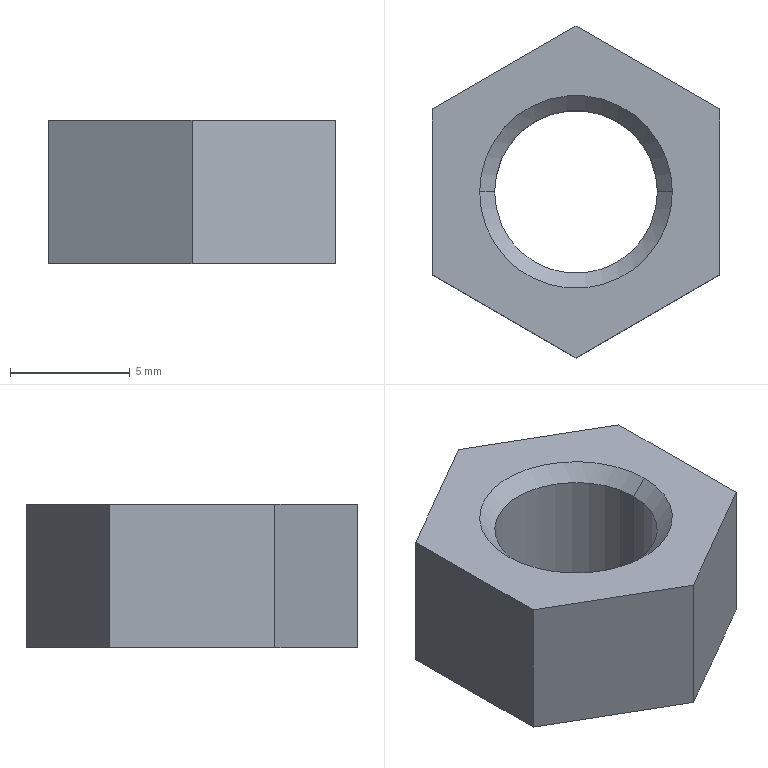Part | SolidWorks | features Extrusion 1, HoleWzd 1 | 1 solid | 12 faces | box 12 x 13.856 x 6 mm | volume 525.917 mm3 | plane 8 | cone 2 | cylinder 2 | commonest cylinder face diameters 6.8 x2
STEP:
#1=CARTESIAN_POINT('',(-2.494,0.7488,5.375));
#2=VERTEX_POINT('',#1);
#3=CARTESIAN_POINT('',(4.306,0.7488,5.375));
#4=VERTEX_POINT('',#3);
#5=CARTESIAN_POINT('',(0.9061,0.7488,5.375));
#6=DIRECTION('',(0.,0.,1.));
#7=DIRECTION('',(1.,0.,0.));
#8=AXIS2_PLACEMENT_3D('',#5,#6,#7);
#9=CIRCLE('',#8,3.4);
#10=EDGE_CURVE('',#2,#4,#9,.T.);
#11=ORIENTED_EDGE('',*,*,#10,.F.);
#12=CARTESIAN_POINT('',(-3.119,0.7488,6.));
#13=VERTEX_POINT('',#12);
#14=CARTESIAN_POINT('',(-3.119,0.7488,6.));
#15=DIRECTION('',(-0.7071,0.,0.7071));
#16=VECTOR('',#15,1000.);
#17=LINE('',#14,#16);
#18=EDGE_CURVE('',#2,#13,#17,.T.);
#19=ORIENTED_EDGE('',*,*,#18,.T.);
#20=CARTESIAN_POINT('',(4.931,0.7488,6.));
#21=VERTEX_POINT('',#20);
#22=CARTESIAN_POINT('',(0.9061,0.7488,6.));
#23=DIRECTION('',(0.,0.,1.));
#24=DIRECTION('',(1.,0.,0.));
#25=AXIS2_PLACEMENT_3D('',#22,#23,#24);
#26=CIRCLE('',#25,4.025);
#27=EDGE_CURVE('',#13,#21,#26,.T.);
#28=ORIENTED_EDGE('',*,*,#27,.T.);
#29=CARTESIAN_POINT('',(4.931,0.7488,6.));
#30=DIRECTION('',(0.7071,0.,0.7071));
#31=VECTOR('',#30,1000.);
#32=LINE('',#29,#31);
#33=EDGE_CURVE('',#4,#21,#32,.T.);
#34=ORIENTED_EDGE('',*,*,#33,.F.);
#35=EDGE_LOOP('',(#11,#19,#28,#34));
#36=FACE_OUTER_BOUND('',#35,.T.);
#37=CARTESIAN_POINT('',(0.9061,0.7488,6.));
#38=DIRECTION('',(0.,0.,1.));
#39=DIRECTION('',(1.,0.,0.));
#40=AXIS2_PLACEMENT_3D('',#37,#38,#39);
#41=CONICAL_SURFACE('',#40,4.025,0.7854);
#42=ADVANCED_FACE('',(#36),#41,.F.);
#43=CARTESIAN_POINT('',(-2.494,0.7488,0.));
#44=VERTEX_POINT('',#43);
#45=CARTESIAN_POINT('',(4.306,0.7488,0.));
#46=VERTEX_POINT('',#45);
#47=CARTESIAN_POINT('',(0.9061,0.7488,0.));
#48=DIRECTION('',(0.,0.,1.));
#49=DIRECTION('',(1.,0.,0.));
#50=AXIS2_PLACEMENT_3D('',#47,#48,#49);
#51=CIRCLE('',#50,3.4);
#52=EDGE_CURVE('',#44,#46,#51,.T.);
#53=ORIENTED_EDGE('',*,*,#52,.F.);
#54=CARTESIAN_POINT('',(-2.494,0.7488,6.));
#55=DIRECTION('',(0.,0.,1.));
#56=VECTOR('',#55,1000.);
#57=LINE('',#54,#56);
#58=EDGE_CURVE('',#44,#2,#57,.T.);
#59=ORIENTED_EDGE('',*,*,#58,.T.);
#60=ORIENTED_EDGE('',*,*,#10,.T.);
#61=CARTESIAN_POINT('',(4.306,0.7488,6.));
#62=DIRECTION('',(0.,0.,1.));
#63=VECTOR('',#62,1000.);
#64=LINE('',#61,#63);
#65=EDGE_CURVE('',#46,#4,#64,.T.);
#66=ORIENTED_EDGE('',*,*,#65,.F.);
#67=EDGE_LOOP('',(#53,#59,#60,#66));
#68=FACE_OUTER_BOUND('',#67,.T.);
#69=CARTESIAN_POINT('',(0.9061,0.7488,6.));
#70=DIRECTION('',(0.,0.,1.));
#71=DIRECTION('',(1.,0.,0.));
#72=AXIS2_PLACEMENT_3D('',#69,#70,#71);
#73=CYLINDRICAL_SURFACE('',#72,3.4);
#74=ADVANCED_FACE('',(#68),#73,.F.);
#75=CARTESIAN_POINT('',(-5.094,-2.715,0.));
#76=VERTEX_POINT('',#75);
#77=CARTESIAN_POINT('',(0.9061,-6.179,0.));
#78=VERTEX_POINT('',#77);
#79=CARTESIAN_POINT('',(0.9061,-6.179,0.));
#80=DIRECTION('',(0.866,-0.5,0.));
#81=VECTOR('',#80,1000.);
#82=LINE('',#79,#81);
#83=EDGE_CURVE('',#76,#78,#82,.T.);
#84=ORIENTED_EDGE('',*,*,#83,.T.);
#85=CARTESIAN_POINT('',(0.9061,-6.179,6.));
#86=VERTEX_POINT('',#85);
#87=CARTESIAN_POINT('',(0.9061,-6.179,6.));
#88=DIRECTION('',(0.,0.,-1.));
#89=VECTOR('',#88,1000.);
#90=LINE('',#87,#89);
#91=EDGE_CURVE('',#86,#78,#90,.T.);
#92=ORIENTED_EDGE('',*,*,#91,.F.);
#93=CARTESIAN_POINT('',(-5.094,-2.715,6.));
#94=VERTEX_POINT('',#93);
#95=CARTESIAN_POINT('',(0.9061,-6.179,6.));
#96=DIRECTION('',(0.866,-0.5,0.));
#97=VECTOR('',#96,1000.);
#98=LINE('',#95,#97);
#99=EDGE_CURVE('',#94,#86,#98,.T.);
#100=ORIENTED_EDGE('',*,*,#99,.F.);
#101=CARTESIAN_POINT('',(-5.094,-2.715,6.));
#102=DIRECTION('',(0.,0.,-1.));
#103=VECTOR('',#102,1000.);
#104=LINE('',#101,#103);
#105=EDGE_CURVE('',#94,#76,#104,.T.);
#106=ORIENTED_EDGE('',*,*,#105,.T.);
#107=EDGE_LOOP('',(#84,#92,#100,#106));
#108=FACE_OUTER_BOUND('',#107,.T.);
#109=CARTESIAN_POINT('',(0.9061,-6.179,6.));
#110=DIRECTION('',(0.5,0.866,0.));
#111=DIRECTION('',(-0.866,0.5,0.));
#112=AXIS2_PLACEMENT_3D('',#109,#110,#111);
#113=PLANE('',#112);
#114=ADVANCED_FACE('',(#108),#113,.F.);
#115=CARTESIAN_POINT('',(6.906,-2.715,0.));
#116=VERTEX_POINT('',#115);
#117=CARTESIAN_POINT('',(6.906,-2.715,0.));
#118=DIRECTION('',(0.866,0.5,0.));
#119=VECTOR('',#118,1000.);
#120=LINE('',#117,#119);
#121=EDGE_CURVE('',#78,#116,#120,.T.);
#122=ORIENTED_EDGE('',*,*,#121,.T.);
#123=CARTESIAN_POINT('',(6.906,-2.715,6.));
#124=VERTEX_POINT('',#123);
#125=CARTESIAN_POINT('',(6.906,-2.715,6.));
#126=DIRECTION('',(0.,0.,-1.));
#127=VECTOR('',#126,1000.);
#128=LINE('',#125,#127);
#129=EDGE_CURVE('',#124,#116,#128,.T.);
#130=ORIENTED_EDGE('',*,*,#129,.F.);
#131=CARTESIAN_POINT('',(6.906,-2.715,6.));
#132=DIRECTION('',(0.866,0.5,0.));
#133=VECTOR('',#132,1000.);
#134=LINE('',#131,#133);
#135=EDGE_CURVE('',#86,#124,#134,.T.);
#136=ORIENTED_EDGE('',*,*,#135,.F.);
#137=ORIENTED_EDGE('',*,*,#91,.T.);
#138=EDGE_LOOP('',(#122,#130,#136,#137));
#139=FACE_OUTER_BOUND('',#138,.T.);
#140=CARTESIAN_POINT('',(6.906,-2.715,6.));
#141=DIRECTION('',(-0.5,0.866,0.));
#142=DIRECTION('',(-0.866,-0.5,0.));
#143=AXIS2_PLACEMENT_3D('',#140,#141,#142);
#144=PLANE('',#143);
#145=ADVANCED_FACE('',(#139),#144,.F.);
#146=CARTESIAN_POINT('',(6.906,4.213,0.));
#147=VERTEX_POINT('',#146);
#148=CARTESIAN_POINT('',(6.906,4.213,0.));
#149=DIRECTION('',(0.,1.,0.));
#150=VECTOR('',#149,1000.);
#151=LINE('',#148,#150);
#152=EDGE_CURVE('',#116,#147,#151,.T.);
#153=ORIENTED_EDGE('',*,*,#152,.T.);
#154=CARTESIAN_POINT('',(6.906,4.213,6.));
#155=VERTEX_POINT('',#154);
#156=CARTESIAN_POINT('',(6.906,4.213,6.));
#157=DIRECTION('',(0.,0.,-1.));
#158=VECTOR('',#157,1000.);
#159=LINE('',#156,#158);
#160=EDGE_CURVE('',#155,#147,#159,.T.);
#161=ORIENTED_EDGE('',*,*,#160,.F.);
#162=CARTESIAN_POINT('',(6.906,4.213,6.));
#163=DIRECTION('',(0.,1.,0.));
#164=VECTOR('',#163,1000.);
#165=LINE('',#162,#164);
#166=EDGE_CURVE('',#124,#155,#165,.T.);
#167=ORIENTED_EDGE('',*,*,#166,.F.);
#168=ORIENTED_EDGE('',*,*,#129,.T.);
#169=EDGE_LOOP('',(#153,#161,#167,#168));
#170=FACE_OUTER_BOUND('',#169,.T.);
#171=CARTESIAN_POINT('',(6.906,4.213,6.));
#172=DIRECTION('',(-1.,0.,0.));
#173=DIRECTION('',(0.,-1.,0.));
#174=AXIS2_PLACEMENT_3D('',#171,#172,#173);
#175=PLANE('',#174);
#176=ADVANCED_FACE('',(#170),#175,.F.);
#177=CARTESIAN_POINT('',(0.9061,7.677,0.));
#178=VERTEX_POINT('',#177);
#179=CARTESIAN_POINT('',(0.9061,7.677,0.));
#180=DIRECTION('',(-0.866,0.5,0.));
#181=VECTOR('',#180,1000.);
#182=LINE('',#179,#181);
#183=EDGE_CURVE('',#147,#178,#182,.T.);
#184=ORIENTED_EDGE('',*,*,#183,.T.);
#185=CARTESIAN_POINT('',(0.9061,7.677,6.));
#186=VERTEX_POINT('',#185);
#187=CARTESIAN_POINT('',(0.9061,7.677,6.));
#188=DIRECTION('',(0.,0.,-1.));
#189=VECTOR('',#188,1000.);
#190=LINE('',#187,#189);
#191=EDGE_CURVE('',#186,#178,#190,.T.);
#192=ORIENTED_EDGE('',*,*,#191,.F.);
#193=CARTESIAN_POINT('',(0.9061,7.677,6.));
#194=DIRECTION('',(-0.866,0.5,0.));
#195=VECTOR('',#194,1000.);
#196=LINE('',#193,#195);
#197=EDGE_CURVE('',#155,#186,#196,.T.);
#198=ORIENTED_EDGE('',*,*,#197,.F.);
#199=ORIENTED_EDGE('',*,*,#160,.T.);
#200=EDGE_LOOP('',(#184,#192,#198,#199));
#201=FACE_OUTER_BOUND('',#200,.T.);
#202=CARTESIAN_POINT('',(0.9061,7.677,6.));
#203=DIRECTION('',(-0.5,-0.866,0.));
#204=DIRECTION('',(0.866,-0.5,0.));
#205=AXIS2_PLACEMENT_3D('',#202,#203,#204);
#206=PLANE('',#205);
#207=ADVANCED_FACE('',(#201),#206,.F.);
#208=CARTESIAN_POINT('',(-5.094,4.213,0.));
#209=VERTEX_POINT('',#208);
#210=CARTESIAN_POINT('',(-5.094,4.213,0.));
#211=DIRECTION('',(-0.866,-0.5,0.));
#212=VECTOR('',#211,1000.);
#213=LINE('',#210,#212);
#214=EDGE_CURVE('',#178,#209,#213,.T.);
#215=ORIENTED_EDGE('',*,*,#214,.T.);
#216=CARTESIAN_POINT('',(-5.094,4.213,6.));
#217=VERTEX_POINT('',#216);
#218=CARTESIAN_POINT('',(-5.094,4.213,6.));
#219=DIRECTION('',(0.,0.,-1.));
#220=VECTOR('',#219,1000.);
#221=LINE('',#218,#220);
#222=EDGE_CURVE('',#217,#209,#221,.T.);
#223=ORIENTED_EDGE('',*,*,#222,.F.);
#224=CARTESIAN_POINT('',(-5.094,4.213,6.));
#225=DIRECTION('',(-0.866,-0.5,0.));
#226=VECTOR('',#225,1000.);
#227=LINE('',#224,#226);
#228=EDGE_CURVE('',#186,#217,#227,.T.);
#229=ORIENTED_EDGE('',*,*,#228,.F.);
#230=ORIENTED_EDGE('',*,*,#191,.T.);
#231=EDGE_LOOP('',(#215,#223,#229,#230));
#232=FACE_OUTER_BOUND('',#231,.T.);
#233=CARTESIAN_POINT('',(-5.094,4.213,6.));
#234=DIRECTION('',(0.5,-0.866,0.));
#235=DIRECTION('',(0.866,0.5,0.));
#236=AXIS2_PLACEMENT_3D('',#233,#234,#235);
#237=PLANE('',#236);
#238=ADVANCED_FACE('',(#232),#237,.F.);
#239=CARTESIAN_POINT('',(-5.094,-2.715,0.));
#240=DIRECTION('',(0.,-1.,0.));
#241=VECTOR('',#240,1000.);
#242=LINE('',#239,#241);
#243=EDGE_CURVE('',#209,#76,#242,.T.);
#244=ORIENTED_EDGE('',*,*,#243,.T.);
#245=ORIENTED_EDGE('',*,*,#105,.F.);
#246=CARTESIAN_POINT('',(-5.094,-2.715,6.));
#247=DIRECTION('',(0.,-1.,0.));
#248=VECTOR('',#247,1000.);
#249=LINE('',#246,#248);
#250=EDGE_CURVE('',#217,#94,#249,.T.);
#251=ORIENTED_EDGE('',*,*,#250,.F.);
#252=ORIENTED_EDGE('',*,*,#222,.T.);
#253=EDGE_LOOP('',(#244,#245,#251,#252));
#254=FACE_OUTER_BOUND('',#253,.T.);
#255=CARTESIAN_POINT('',(-5.094,-2.715,6.));
#256=DIRECTION('',(1.,0.,0.));
#257=DIRECTION('',(0.,1.,0.));
#258=AXIS2_PLACEMENT_3D('',#255,#256,#257);
#259=PLANE('',#258);
#260=ADVANCED_FACE('',(#254),#259,.F.);
#261=CARTESIAN_POINT('',(0.9061,0.7488,6.));
#262=DIRECTION('',(0.,0.,1.));
#263=DIRECTION('',(1.,0.,0.));
#264=AXIS2_PLACEMENT_3D('',#261,#262,#263);
#265=CIRCLE('',#264,4.025);
#266=EDGE_CURVE('',#21,#13,#265,.T.);
#267=ORIENTED_EDGE('',*,*,#266,.F.);
#268=ORIENTED_EDGE('',*,*,#27,.F.);
#269=EDGE_LOOP('',(#267,#268));
#270=FACE_BOUND('',#269,.T.);
#271=ORIENTED_EDGE('',*,*,#99,.T.);
#272=ORIENTED_EDGE('',*,*,#135,.T.);
#273=ORIENTED_EDGE('',*,*,#166,.T.);
#274=ORIENTED_EDGE('',*,*,#197,.T.);
#275=ORIENTED_EDGE('',*,*,#228,.T.);
#276=ORIENTED_EDGE('',*,*,#250,.T.);
#277=EDGE_LOOP('',(#271,#272,#273,#274,#275,#276));
#278=FACE_OUTER_BOUND('',#277,.T.);
#279=CARTESIAN_POINT('',(0.,0.,6.));
#280=DIRECTION('',(0.,0.,-1.));
#281=DIRECTION('',(-1.,0.,0.));
#282=AXIS2_PLACEMENT_3D('',#279,#280,#281);
#283=PLANE('',#282);
#284=ADVANCED_FACE('',(#270,#278),#283,.F.);
#285=CARTESIAN_POINT('',(0.9061,0.7488,0.));
#286=DIRECTION('',(0.,0.,1.));
#287=DIRECTION('',(1.,0.,0.));
#288=AXIS2_PLACEMENT_3D('',#285,#286,#287);
#289=CIRCLE('',#288,3.4);
#290=EDGE_CURVE('',#46,#44,#289,.T.);
#291=ORIENTED_EDGE('',*,*,#290,.T.);
#292=ORIENTED_EDGE('',*,*,#52,.T.);
#293=EDGE_LOOP('',(#291,#292));
#294=FACE_BOUND('',#293,.T.);
#295=ORIENTED_EDGE('',*,*,#83,.F.);
#296=ORIENTED_EDGE('',*,*,#243,.F.);
#297=ORIENTED_EDGE('',*,*,#214,.F.);
#298=ORIENTED_EDGE('',*,*,#183,.F.);
#299=ORIENTED_EDGE('',*,*,#152,.F.);
#300=ORIENTED_EDGE('',*,*,#121,.F.);
#301=EDGE_LOOP('',(#295,#296,#297,#298,#299,#300));
#302=FACE_OUTER_BOUND('',#301,.T.);
#303=CARTESIAN_POINT('',(0.,0.,0.));
#304=DIRECTION('',(0.,0.,-1.));
#305=DIRECTION('',(-1.,0.,0.));
#306=AXIS2_PLACEMENT_3D('',#303,#304,#305);
#307=PLANE('',#306);
#308=ADVANCED_FACE('',(#294,#302),#307,.T.);
#309=ORIENTED_EDGE('',*,*,#58,.F.);
#310=ORIENTED_EDGE('',*,*,#290,.F.);
#311=ORIENTED_EDGE('',*,*,#65,.T.);
#312=CARTESIAN_POINT('',(0.9061,0.7488,5.375));
#313=DIRECTION('',(0.,0.,1.));
#314=DIRECTION('',(1.,0.,0.));
#315=AXIS2_PLACEMENT_3D('',#312,#313,#314);
#316=CIRCLE('',#315,3.4);
#317=EDGE_CURVE('',#4,#2,#316,.T.);
#318=ORIENTED_EDGE('',*,*,#317,.T.);
#319=EDGE_LOOP('',(#309,#310,#311,#318));
#320=FACE_OUTER_BOUND('',#319,.T.);
#321=CARTESIAN_POINT('',(0.9061,0.7488,6.));
#322=DIRECTION('',(0.,0.,1.));
#323=DIRECTION('',(1.,0.,0.));
#324=AXIS2_PLACEMENT_3D('',#321,#322,#323);
#325=CYLINDRICAL_SURFACE('',#324,3.4);
#326=ADVANCED_FACE('',(#320),#325,.F.);
#327=ORIENTED_EDGE('',*,*,#18,.F.);
#328=ORIENTED_EDGE('',*,*,#317,.F.);
#329=ORIENTED_EDGE('',*,*,#33,.T.);
#330=ORIENTED_EDGE('',*,*,#266,.T.);
#331=EDGE_LOOP('',(#327,#328,#329,#330));
#332=FACE_OUTER_BOUND('',#331,.T.);
#333=CARTESIAN_POINT('',(0.9061,0.7488,6.));
#334=DIRECTION('',(0.,0.,1.));
#335=DIRECTION('',(1.,0.,0.));
#336=AXIS2_PLACEMENT_3D('',#333,#334,#335);
#337=CONICAL_SURFACE('',#336,4.025,0.7854);
#338=ADVANCED_FACE('',(#332),#337,.F.);
#339=CLOSED_SHELL('',(#42,#74,#114,#145,#176,#207,#238,#260,#284,#308,#326,#338));
#340=MANIFOLD_SOLID_BREP('',#339);
#341=CARTESIAN_POINT('',(0.,0.,0.));
#342=DIRECTION('',(0.,0.,1.));
#343=DIRECTION('',(1.,0.,0.));
#344=AXIS2_PLACEMENT_3D('',#341,#342,#343);
#345=(LENGTH_UNIT()NAMED_UNIT(*)SI_UNIT(.MILLI.,.METRE.));
#346=UNCERTAINTY_MEASURE_WITH_UNIT(LENGTH_MEASURE(0.00001),#345,'','');
#347=(NAMED_UNIT(*)PLANE_ANGLE_UNIT()SI_UNIT($,.RADIAN.));
#348=(NAMED_UNIT(*)SI_UNIT($,.STERADIAN.)SOLID_ANGLE_UNIT());
#349=(GEOMETRIC_REPRESENTATION_CONTEXT(3)GLOBAL_UNCERTAINTY_ASSIGNED_CONTEXT((#346))GLOBAL_UNIT_ASSIGNED_CONTEXT((#345,#347,#348))REPRESENTATION_CONTEXT('',''));
#350=ADVANCED_BREP_SHAPE_REPRESENTATION('',(#340,#344),#349);